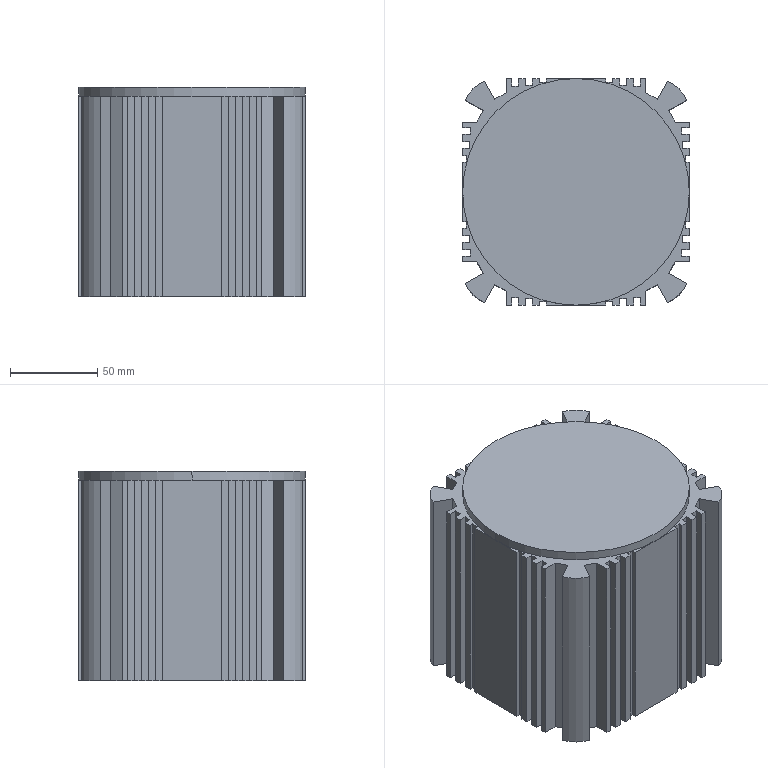Part | SolidWorks | features ICE 3, CirPattern 1, Extrusion 1, Fillet 1, MirrorPattern 1 | 1 solid | 142 faces | box 130 x 130 x 120 mm | volume 1837022 mm3 | plane 132 | cylinder 10 | commonest cylinder face diameters 10 x4 40 x4 130 x2